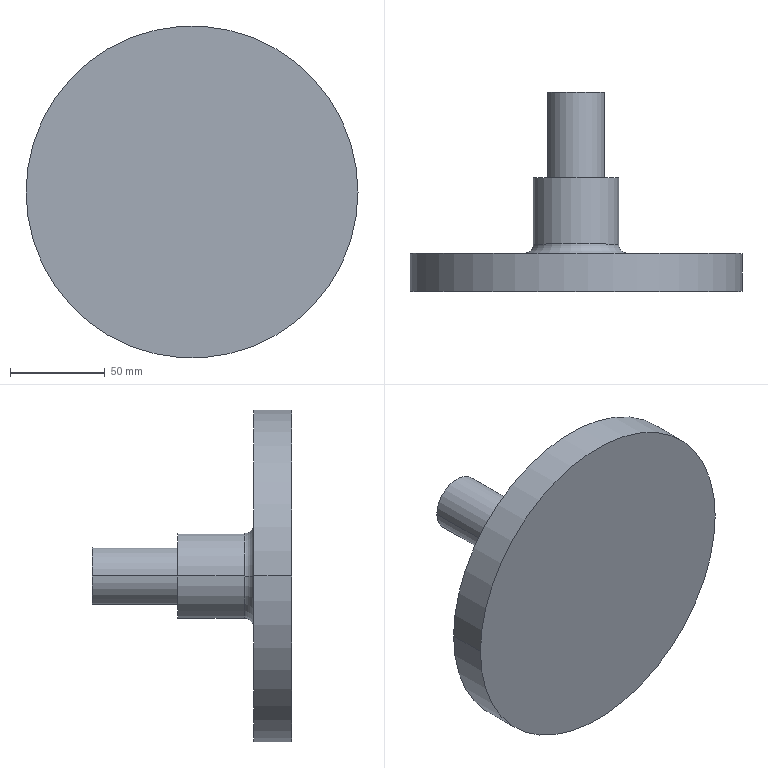Part | STEP file | Roller XG2 | 1 solid | 12 faces | box 175 x 105 x 175 mm | volume 577278 mm3 | cylinder 6 | plane 4 | torus 2 | commonest cylinder face diameters 30 x2 45 x2 175 x2
STEP:
#1=CARTESIAN_POINT('',(0.,0.,0.));
#2=DIRECTION('',(0.,0.,1.));
#3=DIRECTION('',(1.,0.,0.));
#4=AXIS2_PLACEMENT_3D('',#1,#2,#3);
#5=CARTESIAN_POINT('',(-22.5,25.,0.));
#6=VERTEX_POINT('',#5);
#7=CARTESIAN_POINT('',(-27.5,20.,0.));
#8=VERTEX_POINT('',#7);
#9=CARTESIAN_POINT('',(-27.5,25.,0.));
#10=DIRECTION('',(0.,0.,-1.));
#11=DIRECTION('',(-1.,0.,0.));
#12=AXIS2_PLACEMENT_3D('',#9,#10,#11);
#13=CIRCLE('',#12,5.);
#14=CARTESIAN_POINT('',(0.,25.,0.));
#15=DIRECTION('',(0.,1.,0.));
#16=DIRECTION('',(-1.,0.,0.));
#17=AXIS2_PLACEMENT_3D('',#14,#15,#16);
#18=TOROIDAL_SURFACE('',#17,27.5,5.);
#19=CARTESIAN_POINT('',(6.283,0.));
#20=DIRECTION('',(0.,1.));
#21=VECTOR('',#20,1.);
#22=LINE('',#19,#21);
#23=(GEOMETRIC_REPRESENTATION_CONTEXT(2)PARAMETRIC_REPRESENTATION_CONTEXT()REPRESENTATION_CONTEXT('',''));
#24=DEFINITIONAL_REPRESENTATION('',(#22),#23);
#25=PCURVE('',#18,#24);
#26=CARTESIAN_POINT('',(0.,25.,0.));
#27=DIRECTION('',(0.,1.,0.));
#28=DIRECTION('',(-1.,0.,0.));
#29=AXIS2_PLACEMENT_3D('',#26,#27,#28);
#30=TOROIDAL_SURFACE('',#29,27.5,5.);
#31=CARTESIAN_POINT('',(0.,0.));
#32=DIRECTION('',(0.,1.));
#33=VECTOR('',#32,1.);
#34=LINE('',#31,#33);
#35=(GEOMETRIC_REPRESENTATION_CONTEXT(2)PARAMETRIC_REPRESENTATION_CONTEXT()REPRESENTATION_CONTEXT('',''));
#36=DEFINITIONAL_REPRESENTATION('',(#34),#35);
#37=PCURVE('',#30,#36);
#38=SURFACE_CURVE('',#13,(#25,#37),.PCURVE_S1.);
#39=EDGE_CURVE('',#6,#8,#38,.T.);
#40=ORIENTED_EDGE('',*,*,#39,.T.);
#41=CARTESIAN_POINT('',(27.5,20.,0.));
#42=VERTEX_POINT('',#41);
#43=CARTESIAN_POINT('',(0.,20.,0.));
#44=DIRECTION('',(0.,-1.,0.));
#45=DIRECTION('',(-1.,0.,0.));
#46=AXIS2_PLACEMENT_3D('',#43,#44,#45);
#47=CIRCLE('',#46,27.5);
#48=CARTESIAN_POINT('',(6.283,4.712));
#49=DIRECTION('',(-1.,0.));
#50=VECTOR('',#49,1.);
#51=LINE('',#48,#50);
#52=(GEOMETRIC_REPRESENTATION_CONTEXT(2)PARAMETRIC_REPRESENTATION_CONTEXT()REPRESENTATION_CONTEXT('',''));
#53=DEFINITIONAL_REPRESENTATION('',(#51),#52);
#54=PCURVE('',#18,#53);
#55=CARTESIAN_POINT('',(87.5,20.,0.));
#56=DIRECTION('',(0.,1.,0.));
#57=DIRECTION('',(-1.,0.,0.));
#58=AXIS2_PLACEMENT_3D('',#55,#56,#57);
#59=PLANE('',#58);
#60=CARTESIAN_POINT('',(115.,0.));
#61=CARTESIAN_POINT('',(115.,-47.631));
#62=CARTESIAN_POINT('',(73.75,-23.816));
#63=CARTESIAN_POINT('',(32.5,0.));
#64=CARTESIAN_POINT('',(73.75,23.816));
#65=CARTESIAN_POINT('',(115.,47.631));
#66=CARTESIAN_POINT('',(115.,0.));
#67=(BOUNDED_CURVE()B_SPLINE_CURVE(2,(#60,#61,#62,#63,#64,#65,#66),.UNSPECIFIED.,.T.,.F.)B_SPLINE_CURVE_WITH_KNOTS((1,2,2,2,2,1),(-2.094,0.,2.094,4.189,6.283,8.378),.UNSPECIFIED.)CURVE()GEOMETRIC_REPRESENTATION_ITEM()RATIONAL_B_SPLINE_CURVE((1.,0.5,1.,0.5,1.,0.5,1.))REPRESENTATION_ITEM(''));
#68=(GEOMETRIC_REPRESENTATION_CONTEXT(2)PARAMETRIC_REPRESENTATION_CONTEXT()REPRESENTATION_CONTEXT('',''));
#69=DEFINITIONAL_REPRESENTATION('',(#67),#68);
#70=PCURVE('',#59,#69);
#71=SURFACE_CURVE('',#47,(#54,#70),.PCURVE_S1.);
#72=EDGE_CURVE('',#8,#42,#71,.T.);
#73=ORIENTED_EDGE('',*,*,#72,.T.);
#74=CARTESIAN_POINT('',(22.5,25.,0.));
#75=VERTEX_POINT('',#74);
#76=CARTESIAN_POINT('',(27.5,25.,0.));
#77=DIRECTION('',(0.,0.,1.));
#78=DIRECTION('',(1.,0.,0.));
#79=AXIS2_PLACEMENT_3D('',#76,#77,#78);
#80=CIRCLE('',#79,5.);
#81=CARTESIAN_POINT('',(3.142,0.));
#82=DIRECTION('',(0.,1.));
#83=VECTOR('',#82,1.);
#84=LINE('',#81,#83);
#85=(GEOMETRIC_REPRESENTATION_CONTEXT(2)PARAMETRIC_REPRESENTATION_CONTEXT()REPRESENTATION_CONTEXT('',''));
#86=DEFINITIONAL_REPRESENTATION('',(#84),#85);
#87=PCURVE('',#18,#86);
#88=CARTESIAN_POINT('',(3.142,0.));
#89=DIRECTION('',(0.,1.));
#90=VECTOR('',#89,1.);
#91=LINE('',#88,#90);
#92=(GEOMETRIC_REPRESENTATION_CONTEXT(2)PARAMETRIC_REPRESENTATION_CONTEXT()REPRESENTATION_CONTEXT('',''));
#93=DEFINITIONAL_REPRESENTATION('',(#91),#92);
#94=PCURVE('',#30,#93);
#95=SURFACE_CURVE('',#80,(#87,#94),.PCURVE_S1.);
#96=EDGE_CURVE('',#75,#42,#95,.T.);
#97=ORIENTED_EDGE('',*,*,#96,.F.);
#98=CARTESIAN_POINT('',(0.,25.,0.));
#99=DIRECTION('',(0.,1.,0.));
#100=DIRECTION('',(-1.,0.,0.));
#101=AXIS2_PLACEMENT_3D('',#98,#99,#100);
#102=CIRCLE('',#101,22.5);
#103=CARTESIAN_POINT('',(0.,3.142));
#104=DIRECTION('',(1.,0.));
#105=VECTOR('',#104,1.);
#106=LINE('',#103,#105);
#107=(GEOMETRIC_REPRESENTATION_CONTEXT(2)PARAMETRIC_REPRESENTATION_CONTEXT()REPRESENTATION_CONTEXT('',''));
#108=DEFINITIONAL_REPRESENTATION('',(#106),#107);
#109=PCURVE('',#18,#108);
#110=CARTESIAN_POINT('',(0.,-777.265,0.));
#111=DIRECTION('',(0.,-1.,0.));
#112=DIRECTION('',(1.,0.,0.));
#113=AXIS2_PLACEMENT_3D('',#110,#111,#112);
#114=CYLINDRICAL_SURFACE('',#113,22.5);
#115=CARTESIAN_POINT('',(9.425,-802.265));
#116=DIRECTION('',(-1.,0.));
#117=VECTOR('',#116,1.);
#118=LINE('',#115,#117);
#119=(GEOMETRIC_REPRESENTATION_CONTEXT(2)PARAMETRIC_REPRESENTATION_CONTEXT()REPRESENTATION_CONTEXT('',''));
#120=DEFINITIONAL_REPRESENTATION('',(#118),#119);
#121=PCURVE('',#114,#120);
#122=SURFACE_CURVE('',#102,(#109,#121),.PCURVE_S1.);
#123=EDGE_CURVE('',#75,#6,#122,.T.);
#124=ORIENTED_EDGE('',*,*,#123,.T.);
#125=EDGE_LOOP('',(#40,#73,#97,#124));
#126=FACE_BOUND('',#125,.F.);
#127=ADVANCED_FACE('',(#126),#18,.F.);
#128=CARTESIAN_POINT('',(15.,105.,0.));
#129=VERTEX_POINT('',#128);
#130=CARTESIAN_POINT('',(-15.,105.,0.));
#131=VERTEX_POINT('',#130);
#132=CARTESIAN_POINT('',(0.,105.,0.));
#133=DIRECTION('',(0.,-1.,0.));
#134=DIRECTION('',(1.,0.,0.));
#135=AXIS2_PLACEMENT_3D('',#132,#133,#134);
#136=CIRCLE('',#135,15.);
#137=CARTESIAN_POINT('',(0.,-777.265,0.));
#138=DIRECTION('',(0.,-1.,0.));
#139=DIRECTION('',(1.,0.,0.));
#140=AXIS2_PLACEMENT_3D('',#137,#138,#139);
#141=CYLINDRICAL_SURFACE('',#140,15.);
#142=CARTESIAN_POINT('',(0.,-882.265));
#143=DIRECTION('',(1.,0.));
#144=VECTOR('',#143,1.);
#145=LINE('',#142,#144);
#146=(GEOMETRIC_REPRESENTATION_CONTEXT(2)PARAMETRIC_REPRESENTATION_CONTEXT()REPRESENTATION_CONTEXT('',''));
#147=DEFINITIONAL_REPRESENTATION('',(#145),#146);
#148=PCURVE('',#141,#147);
#149=CARTESIAN_POINT('',(15.,105.,0.));
#150=DIRECTION('',(0.,1.,0.));
#151=DIRECTION('',(-1.,0.,0.));
#152=AXIS2_PLACEMENT_3D('',#149,#150,#151);
#153=PLANE('',#152);
#154=CARTESIAN_POINT('',(0.,0.));
#155=CARTESIAN_POINT('',(0.,25.981));
#156=CARTESIAN_POINT('',(22.5,12.99));
#157=CARTESIAN_POINT('',(45.,0.));
#158=CARTESIAN_POINT('',(22.5,-12.99));
#159=CARTESIAN_POINT('',(0.,-25.981));
#160=CARTESIAN_POINT('',(0.,0.));
#161=(BOUNDED_CURVE()B_SPLINE_CURVE(2,(#154,#155,#156,#157,#158,#159,#160),.UNSPECIFIED.,.T.,.F.)B_SPLINE_CURVE_WITH_KNOTS((1,2,2,2,2,1),(-2.094,0.,2.094,4.189,6.283,8.378),.UNSPECIFIED.)CURVE()GEOMETRIC_REPRESENTATION_ITEM()RATIONAL_B_SPLINE_CURVE((1.,0.5,1.,0.5,1.,0.5,1.))REPRESENTATION_ITEM(''));
#162=(GEOMETRIC_REPRESENTATION_CONTEXT(2)PARAMETRIC_REPRESENTATION_CONTEXT()REPRESENTATION_CONTEXT('',''));
#163=DEFINITIONAL_REPRESENTATION('',(#161),#162);
#164=PCURVE('',#153,#163);
#165=SURFACE_CURVE('',#136,(#148,#164),.PCURVE_S1.);
#166=EDGE_CURVE('',#129,#131,#165,.T.);
#167=ORIENTED_EDGE('',*,*,#166,.T.);
#168=CARTESIAN_POINT('',(-15.,60.,0.));
#169=VERTEX_POINT('',#168);
#170=CARTESIAN_POINT('',(-15.,-777.265,0.));
#171=DIRECTION('',(0.,-1.,0.));
#172=VECTOR('',#171,1.);
#173=LINE('',#170,#172);
#174=CARTESIAN_POINT('',(3.142,0.));
#175=DIRECTION('',(0.,1.));
#176=VECTOR('',#175,1.);
#177=LINE('',#174,#176);
#178=(GEOMETRIC_REPRESENTATION_CONTEXT(2)PARAMETRIC_REPRESENTATION_CONTEXT()REPRESENTATION_CONTEXT('',''));
#179=DEFINITIONAL_REPRESENTATION('',(#177),#178);
#180=PCURVE('',#141,#179);
#181=CARTESIAN_POINT('',(0.,-777.265,0.));
#182=DIRECTION('',(0.,-1.,0.));
#183=DIRECTION('',(1.,0.,0.));
#184=AXIS2_PLACEMENT_3D('',#181,#182,#183);
#185=CYLINDRICAL_SURFACE('',#184,15.);
#186=CARTESIAN_POINT('',(3.142,0.));
#187=DIRECTION('',(0.,1.));
#188=VECTOR('',#187,1.);
#189=LINE('',#186,#188);
#190=(GEOMETRIC_REPRESENTATION_CONTEXT(2)PARAMETRIC_REPRESENTATION_CONTEXT()REPRESENTATION_CONTEXT('',''));
#191=DEFINITIONAL_REPRESENTATION('',(#189),#190);
#192=PCURVE('',#185,#191);
#193=SURFACE_CURVE('',#173,(#180,#192),.PCURVE_S1.);
#194=EDGE_CURVE('',#131,#169,#193,.T.);
#195=ORIENTED_EDGE('',*,*,#194,.T.);
#196=CARTESIAN_POINT('',(15.,60.,0.));
#197=VERTEX_POINT('',#196);
#198=CARTESIAN_POINT('',(0.,60.,0.));
#199=DIRECTION('',(0.,-1.,0.));
#200=DIRECTION('',(1.,0.,0.));
#201=AXIS2_PLACEMENT_3D('',#198,#199,#200);
#202=CIRCLE('',#201,15.);
#203=CARTESIAN_POINT('',(0.,-837.265));
#204=DIRECTION('',(1.,0.));
#205=VECTOR('',#204,1.);
#206=LINE('',#203,#205);
#207=(GEOMETRIC_REPRESENTATION_CONTEXT(2)PARAMETRIC_REPRESENTATION_CONTEXT()REPRESENTATION_CONTEXT('',''));
#208=DEFINITIONAL_REPRESENTATION('',(#206),#207);
#209=PCURVE('',#141,#208);
#210=CARTESIAN_POINT('',(22.5,60.,0.));
#211=DIRECTION('',(0.,1.,0.));
#212=DIRECTION('',(-1.,0.,0.));
#213=AXIS2_PLACEMENT_3D('',#210,#211,#212);
#214=PLANE('',#213);
#215=CARTESIAN_POINT('',(7.5,0.));
#216=CARTESIAN_POINT('',(7.5,25.981));
#217=CARTESIAN_POINT('',(30.,12.99));
#218=CARTESIAN_POINT('',(52.5,0.));
#219=CARTESIAN_POINT('',(30.,-12.99));
#220=CARTESIAN_POINT('',(7.5,-25.981));
#221=CARTESIAN_POINT('',(7.5,0.));
#222=(BOUNDED_CURVE()B_SPLINE_CURVE(2,(#215,#216,#217,#218,#219,#220,#221),.UNSPECIFIED.,.T.,.F.)B_SPLINE_CURVE_WITH_KNOTS((1,2,2,2,2,1),(-2.094,0.,2.094,4.189,6.283,8.378),.UNSPECIFIED.)CURVE()GEOMETRIC_REPRESENTATION_ITEM()RATIONAL_B_SPLINE_CURVE((1.,0.5,1.,0.5,1.,0.5,1.))REPRESENTATION_ITEM(''));
#223=(GEOMETRIC_REPRESENTATION_CONTEXT(2)PARAMETRIC_REPRESENTATION_CONTEXT()REPRESENTATION_CONTEXT('',''));
#224=DEFINITIONAL_REPRESENTATION('',(#222),#223);
#225=PCURVE('',#214,#224);
#226=SURFACE_CURVE('',#202,(#209,#225),.PCURVE_S1.);
#227=EDGE_CURVE('',#197,#169,#226,.T.);
#228=ORIENTED_EDGE('',*,*,#227,.F.);
#229=CARTESIAN_POINT('',(15.,-777.265,0.));
#230=DIRECTION('',(0.,-1.,0.));
#231=VECTOR('',#230,1.);
#232=LINE('',#229,#231);
#233=CARTESIAN_POINT('',(0.,0.));
#234=DIRECTION('',(0.,1.));
#235=VECTOR('',#234,1.);
#236=LINE('',#233,#235);
#237=(GEOMETRIC_REPRESENTATION_CONTEXT(2)PARAMETRIC_REPRESENTATION_CONTEXT()REPRESENTATION_CONTEXT('',''));
#238=DEFINITIONAL_REPRESENTATION('',(#236),#237);
#239=PCURVE('',#141,#238);
#240=CARTESIAN_POINT('',(6.283,0.));
#241=DIRECTION('',(0.,1.));
#242=VECTOR('',#241,1.);
#243=LINE('',#240,#242);
#244=(GEOMETRIC_REPRESENTATION_CONTEXT(2)PARAMETRIC_REPRESENTATION_CONTEXT()REPRESENTATION_CONTEXT('',''));
#245=DEFINITIONAL_REPRESENTATION('',(#243),#244);
#246=PCURVE('',#185,#245);
#247=SURFACE_CURVE('',#232,(#239,#246),.PCURVE_S1.);
#248=EDGE_CURVE('',#129,#197,#247,.T.);
#249=ORIENTED_EDGE('',*,*,#248,.F.);
#250=EDGE_LOOP('',(#167,#195,#228,#249));
#251=FACE_BOUND('',#250,.T.);
#252=ADVANCED_FACE('',(#251),#141,.T.);
#253=CARTESIAN_POINT('',(22.5,60.,0.));
#254=VERTEX_POINT('',#253);
#255=CARTESIAN_POINT('',(-22.5,60.,0.));
#256=VERTEX_POINT('',#255);
#257=CARTESIAN_POINT('',(0.,60.,0.));
#258=DIRECTION('',(0.,-1.,0.));
#259=DIRECTION('',(1.,0.,0.));
#260=AXIS2_PLACEMENT_3D('',#257,#258,#259);
#261=CIRCLE('',#260,22.5);
#262=CARTESIAN_POINT('',(0.,-777.265,0.));
#263=DIRECTION('',(0.,-1.,0.));
#264=DIRECTION('',(1.,0.,0.));
#265=AXIS2_PLACEMENT_3D('',#262,#263,#264);
#266=CYLINDRICAL_SURFACE('',#265,22.5);
#267=CARTESIAN_POINT('',(0.,-837.265));
#268=DIRECTION('',(1.,0.));
#269=VECTOR('',#268,1.);
#270=LINE('',#267,#269);
#271=(GEOMETRIC_REPRESENTATION_CONTEXT(2)PARAMETRIC_REPRESENTATION_CONTEXT()REPRESENTATION_CONTEXT('',''));
#272=DEFINITIONAL_REPRESENTATION('',(#270),#271);
#273=PCURVE('',#266,#272);
#274=CARTESIAN_POINT('',(0.,0.));
#275=CARTESIAN_POINT('',(0.,38.971));
#276=CARTESIAN_POINT('',(33.75,19.486));
#277=CARTESIAN_POINT('',(67.5,0.));
#278=CARTESIAN_POINT('',(33.75,-19.486));
#279=CARTESIAN_POINT('',(0.,-38.971));
#280=CARTESIAN_POINT('',(0.,0.));
#281=(BOUNDED_CURVE()B_SPLINE_CURVE(2,(#274,#275,#276,#277,#278,#279,#280),.UNSPECIFIED.,.T.,.F.)B_SPLINE_CURVE_WITH_KNOTS((1,2,2,2,2,1),(-2.094,0.,2.094,4.189,6.283,8.378),.UNSPECIFIED.)CURVE()GEOMETRIC_REPRESENTATION_ITEM()RATIONAL_B_SPLINE_CURVE((1.,0.5,1.,0.5,1.,0.5,1.))REPRESENTATION_ITEM(''));
#282=(GEOMETRIC_REPRESENTATION_CONTEXT(2)PARAMETRIC_REPRESENTATION_CONTEXT()REPRESENTATION_CONTEXT('',''));
#283=DEFINITIONAL_REPRESENTATION('',(#281),#282);
#284=PCURVE('',#214,#283);
#285=SURFACE_CURVE('',#261,(#273,#284),.PCURVE_S1.);
#286=EDGE_CURVE('',#254,#256,#285,.T.);
#287=ORIENTED_EDGE('',*,*,#286,.T.);
#288=CARTESIAN_POINT('',(-22.5,-777.265,0.));
#289=DIRECTION('',(0.,-1.,0.));
#290=VECTOR('',#289,1.);
#291=LINE('',#288,#290);
#292=CARTESIAN_POINT('',(3.142,0.));
#293=DIRECTION('',(0.,1.));
#294=VECTOR('',#293,1.);
#295=LINE('',#292,#294);
#296=(GEOMETRIC_REPRESENTATION_CONTEXT(2)PARAMETRIC_REPRESENTATION_CONTEXT()REPRESENTATION_CONTEXT('',''));
#297=DEFINITIONAL_REPRESENTATION('',(#295),#296);
#298=PCURVE('',#266,#297);
#299=CARTESIAN_POINT('',(3.142,0.));
#300=DIRECTION('',(0.,1.));
#301=VECTOR('',#300,1.);
#302=LINE('',#299,#301);
#303=(GEOMETRIC_REPRESENTATION_CONTEXT(2)PARAMETRIC_REPRESENTATION_CONTEXT()REPRESENTATION_CONTEXT('',''));
#304=DEFINITIONAL_REPRESENTATION('',(#302),#303);
#305=PCURVE('',#114,#304);
#306=SURFACE_CURVE('',#291,(#298,#305),.PCURVE_S1.);
#307=EDGE_CURVE('',#256,#6,#306,.T.);
#308=ORIENTED_EDGE('',*,*,#307,.T.);
#309=CARTESIAN_POINT('',(0.,25.,0.));
#310=DIRECTION('',(0.,1.,0.));
#311=DIRECTION('',(-1.,0.,0.));
#312=AXIS2_PLACEMENT_3D('',#309,#310,#311);
#313=CIRCLE('',#312,22.5);
#314=CARTESIAN_POINT('',(3.142,-802.265));
#315=DIRECTION('',(-1.,0.));
#316=VECTOR('',#315,1.);
#317=LINE('',#314,#316);
#318=(GEOMETRIC_REPRESENTATION_CONTEXT(2)PARAMETRIC_REPRESENTATION_CONTEXT()REPRESENTATION_CONTEXT('',''));
#319=DEFINITIONAL_REPRESENTATION('',(#317),#318);
#320=PCURVE('',#266,#319);
#321=CARTESIAN_POINT('',(0.,3.142));
#322=DIRECTION('',(1.,0.));
#323=VECTOR('',#322,1.);
#324=LINE('',#321,#323);
#325=(GEOMETRIC_REPRESENTATION_CONTEXT(2)PARAMETRIC_REPRESENTATION_CONTEXT()REPRESENTATION_CONTEXT('',''));
#326=DEFINITIONAL_REPRESENTATION('',(#324),#325);
#327=PCURVE('',#30,#326);
#328=SURFACE_CURVE('',#313,(#320,#327),.PCURVE_S1.);
#329=EDGE_CURVE('',#6,#75,#328,.T.);
#330=ORIENTED_EDGE('',*,*,#329,.T.);
#331=CARTESIAN_POINT('',(22.5,-777.265,0.));
#332=DIRECTION('',(0.,-1.,0.));
#333=VECTOR('',#332,1.);
#334=LINE('',#331,#333);
#335=CARTESIAN_POINT('',(0.,0.));
#336=DIRECTION('',(0.,1.));
#337=VECTOR('',#336,1.);
#338=LINE('',#335,#337);
#339=(GEOMETRIC_REPRESENTATION_CONTEXT(2)PARAMETRIC_REPRESENTATION_CONTEXT()REPRESENTATION_CONTEXT('',''));
#340=DEFINITIONAL_REPRESENTATION('',(#338),#339);
#341=PCURVE('',#266,#340);
#342=CARTESIAN_POINT('',(6.283,0.));
#343=DIRECTION('',(0.,1.));
#344=VECTOR('',#343,1.);
#345=LINE('',#342,#344);
#346=(GEOMETRIC_REPRESENTATION_CONTEXT(2)PARAMETRIC_REPRESENTATION_CONTEXT()REPRESENTATION_CONTEXT('',''));
#347=DEFINITIONAL_REPRESENTATION('',(#345),#346);
#348=PCURVE('',#114,#347);
#349=SURFACE_CURVE('',#334,(#341,#348),.PCURVE_S1.);
#350=EDGE_CURVE('',#254,#75,#349,.T.);
#351=ORIENTED_EDGE('',*,*,#350,.F.);
#352=EDGE_LOOP('',(#287,#308,#330,#351));
#353=FACE_BOUND('',#352,.T.);
#354=ADVANCED_FACE('',(#353),#266,.T.);
#355=CARTESIAN_POINT('',(87.5,20.,0.));
#356=VERTEX_POINT('',#355);
#357=CARTESIAN_POINT('',(-87.5,20.,0.));
#358=VERTEX_POINT('',#357);
#359=CARTESIAN_POINT('',(0.,20.,0.));
#360=DIRECTION('',(0.,-1.,0.));
#361=DIRECTION('',(1.,0.,0.));
#362=AXIS2_PLACEMENT_3D('',#359,#360,#361);
#363=CIRCLE('',#362,87.5);
#364=CARTESIAN_POINT('',(0.,-777.265,0.));
#365=DIRECTION('',(0.,-1.,0.));
#366=DIRECTION('',(1.,0.,0.));
#367=AXIS2_PLACEMENT_3D('',#364,#365,#366);
#368=CYLINDRICAL_SURFACE('',#367,87.5);
#369=CARTESIAN_POINT('',(0.,-797.265));
#370=DIRECTION('',(1.,0.));
#371=VECTOR('',#370,1.);
#372=LINE('',#369,#371);
#373=(GEOMETRIC_REPRESENTATION_CONTEXT(2)PARAMETRIC_REPRESENTATION_CONTEXT()REPRESENTATION_CONTEXT('',''));
#374=DEFINITIONAL_REPRESENTATION('',(#372),#373);
#375=PCURVE('',#368,#374);
#376=CARTESIAN_POINT('',(0.,0.));
#377=CARTESIAN_POINT('',(0.,151.554));
#378=CARTESIAN_POINT('',(131.25,75.777));
#379=CARTESIAN_POINT('',(262.5,0.));
#380=CARTESIAN_POINT('',(131.25,-75.777));
#381=CARTESIAN_POINT('',(0.,-151.554));
#382=CARTESIAN_POINT('',(0.,0.));
#383=(BOUNDED_CURVE()B_SPLINE_CURVE(2,(#376,#377,#378,#379,#380,#381,#382),.UNSPECIFIED.,.T.,.F.)B_SPLINE_CURVE_WITH_KNOTS((1,2,2,2,2,1),(-2.094,0.,2.094,4.189,6.283,8.378),.UNSPECIFIED.)CURVE()GEOMETRIC_REPRESENTATION_ITEM()RATIONAL_B_SPLINE_CURVE((1.,0.5,1.,0.5,1.,0.5,1.))REPRESENTATION_ITEM(''));
#384=(GEOMETRIC_REPRESENTATION_CONTEXT(2)PARAMETRIC_REPRESENTATION_CONTEXT()REPRESENTATION_CONTEXT('',''));
#385=DEFINITIONAL_REPRESENTATION('',(#383),#384);
#386=PCURVE('',#59,#385);
#387=SURFACE_CURVE('',#363,(#375,#386),.PCURVE_S1.);
#388=EDGE_CURVE('',#356,#358,#387,.T.);
#389=ORIENTED_EDGE('',*,*,#388,.T.);
#390=CARTESIAN_POINT('',(-87.5,0.,0.));
#391=VERTEX_POINT('',#390);
#392=CARTESIAN_POINT('',(-87.5,-777.265,0.));
#393=DIRECTION('',(0.,-1.,0.));
#394=VECTOR('',#393,1.);
#395=LINE('',#392,#394);
#396=CARTESIAN_POINT('',(3.142,0.));
#397=DIRECTION('',(0.,1.));
#398=VECTOR('',#397,1.);
#399=LINE('',#396,#398);
#400=(GEOMETRIC_REPRESENTATION_CONTEXT(2)PARAMETRIC_REPRESENTATION_CONTEXT()REPRESENTATION_CONTEXT('',''));
#401=DEFINITIONAL_REPRESENTATION('',(#399),#400);
#402=PCURVE('',#368,#401);
#403=CARTESIAN_POINT('',(0.,-777.265,0.));
#404=DIRECTION('',(0.,-1.,0.));
#405=DIRECTION('',(1.,0.,0.));
#406=AXIS2_PLACEMENT_3D('',#403,#404,#405);
#407=CYLINDRICAL_SURFACE('',#406,87.5);
#408=CARTESIAN_POINT('',(3.142,0.));
#409=DIRECTION('',(0.,1.));
#410=VECTOR('',#409,1.);
#411=LINE('',#408,#410);
#412=(GEOMETRIC_REPRESENTATION_CONTEXT(2)PARAMETRIC_REPRESENTATION_CONTEXT()REPRESENTATION_CONTEXT('',''));
#413=DEFINITIONAL_REPRESENTATION('',(#411),#412);
#414=PCURVE('',#407,#413);
#415=SURFACE_CURVE('',#395,(#402,#414),.PCURVE_S1.);
#416=EDGE_CURVE('',#358,#391,#415,.T.);
#417=ORIENTED_EDGE('',*,*,#416,.T.);
#418=CARTESIAN_POINT('',(87.5,0.,0.));
#419=VERTEX_POINT('',#418);
#420=CARTESIAN_POINT('',(0.,0.,0.));
#421=DIRECTION('',(0.,-1.,0.));
#422=DIRECTION('',(1.,0.,0.));
#423=AXIS2_PLACEMENT_3D('',#420,#421,#422);
#424=CIRCLE('',#423,87.5);
#425=CARTESIAN_POINT('',(0.,-777.265));
#426=DIRECTION('',(1.,0.));
#427=VECTOR('',#426,1.);
#428=LINE('',#425,#427);
#429=(GEOMETRIC_REPRESENTATION_CONTEXT(2)PARAMETRIC_REPRESENTATION_CONTEXT()REPRESENTATION_CONTEXT('',''));
#430=DEFINITIONAL_REPRESENTATION('',(#428),#429);
#431=PCURVE('',#368,#430);
#432=CARTESIAN_POINT('',(87.5,0.,0.));
#433=DIRECTION('',(0.,-1.,0.));
#434=DIRECTION('',(1.,0.,0.));
#435=AXIS2_PLACEMENT_3D('',#432,#433,#434);
#436=PLANE('',#435);
#437=CARTESIAN_POINT('',(-87.5,0.));
#438=DIRECTION('',(1.,0.));
#439=AXIS2_PLACEMENT_2D('',#437,#438);
#440=CIRCLE('',#439,87.5);
#441=(GEOMETRIC_REPRESENTATION_CONTEXT(2)PARAMETRIC_REPRESENTATION_CONTEXT()REPRESENTATION_CONTEXT('',''));
#442=DEFINITIONAL_REPRESENTATION('',(#440),#441);
#443=PCURVE('',#436,#442);
#444=SURFACE_CURVE('',#424,(#431,#443),.PCURVE_S1.);
#445=EDGE_CURVE('',#419,#391,#444,.T.);
#446=ORIENTED_EDGE('',*,*,#445,.F.);
#447=CARTESIAN_POINT('',(87.5,-777.265,0.));
#448=DIRECTION('',(0.,-1.,0.));
#449=VECTOR('',#448,1.);
#450=LINE('',#447,#449);
#451=CARTESIAN_POINT('',(0.,0.));
#452=DIRECTION('',(0.,1.));
#453=VECTOR('',#452,1.);
#454=LINE('',#451,#453);
#455=(GEOMETRIC_REPRESENTATION_CONTEXT(2)PARAMETRIC_REPRESENTATION_CONTEXT()REPRESENTATION_CONTEXT('',''));
#456=DEFINITIONAL_REPRESENTATION('',(#454),#455);
#457=PCURVE('',#368,#456);
#458=CARTESIAN_POINT('',(6.283,0.));
#459=DIRECTION('',(0.,1.));
#460=VECTOR('',#459,1.);
#461=LINE('',#458,#460);
#462=(GEOMETRIC_REPRESENTATION_CONTEXT(2)PARAMETRIC_REPRESENTATION_CONTEXT()REPRESENTATION_CONTEXT('',''));
#463=DEFINITIONAL_REPRESENTATION('',(#461),#462);
#464=PCURVE('',#407,#463);
#465=SURFACE_CURVE('',#450,(#457,#464),.PCURVE_S1.);
#466=EDGE_CURVE('',#356,#419,#465,.T.);
#467=ORIENTED_EDGE('',*,*,#466,.F.);
#468=EDGE_LOOP('',(#389,#417,#446,#467));
#469=FACE_BOUND('',#468,.T.);
#470=ADVANCED_FACE('',(#469),#368,.T.);
#471=ORIENTED_EDGE('',*,*,#416,.F.);
#472=CARTESIAN_POINT('',(0.,20.,0.));
#473=DIRECTION('',(0.,-1.,0.));
#474=DIRECTION('',(1.,0.,0.));
#475=AXIS2_PLACEMENT_3D('',#472,#473,#474);
#476=CIRCLE('',#475,87.5);
#477=CARTESIAN_POINT('',(0.,-797.265));
#478=DIRECTION('',(1.,0.));
#479=VECTOR('',#478,1.);
#480=LINE('',#477,#479);
#481=(GEOMETRIC_REPRESENTATION_CONTEXT(2)PARAMETRIC_REPRESENTATION_CONTEXT()REPRESENTATION_CONTEXT('',''));
#482=DEFINITIONAL_REPRESENTATION('',(#480),#481);
#483=PCURVE('',#407,#482);
#484=CARTESIAN_POINT('',(0.,0.));
#485=CARTESIAN_POINT('',(0.,151.554));
#486=CARTESIAN_POINT('',(131.25,75.777));
#487=CARTESIAN_POINT('',(262.5,0.));
#488=CARTESIAN_POINT('',(131.25,-75.777));
#489=CARTESIAN_POINT('',(0.,-151.554));
#490=CARTESIAN_POINT('',(0.,0.));
#491=(BOUNDED_CURVE()B_SPLINE_CURVE(2,(#484,#485,#486,#487,#488,#489,#490),.UNSPECIFIED.,.T.,.F.)B_SPLINE_CURVE_WITH_KNOTS((1,2,2,2,2,1),(-2.094,0.,2.094,4.189,6.283,8.378),.UNSPECIFIED.)CURVE()GEOMETRIC_REPRESENTATION_ITEM()RATIONAL_B_SPLINE_CURVE((1.,0.5,1.,0.5,1.,0.5,1.))REPRESENTATION_ITEM(''));
#492=(GEOMETRIC_REPRESENTATION_CONTEXT(2)PARAMETRIC_REPRESENTATION_CONTEXT()REPRESENTATION_CONTEXT('',''));
#493=DEFINITIONAL_REPRESENTATION('',(#491),#492);
#494=PCURVE('',#59,#493);
#495=SURFACE_CURVE('',#476,(#483,#494),.PCURVE_S1.);
#496=EDGE_CURVE('',#358,#356,#495,.T.);
#497=ORIENTED_EDGE('',*,*,#496,.T.);
#498=ORIENTED_EDGE('',*,*,#466,.T.);
#499=CARTESIAN_POINT('',(0.,0.,0.));
#500=DIRECTION('',(0.,-1.,0.));
#501=DIRECTION('',(1.,0.,0.));
#502=AXIS2_PLACEMENT_3D('',#499,#500,#501);
#503=CIRCLE('',#502,87.5);
#504=CARTESIAN_POINT('',(0.,-777.265));
#505=DIRECTION('',(1.,0.));
#506=VECTOR('',#505,1.);
#507=LINE('',#504,#506);
#508=(GEOMETRIC_REPRESENTATION_CONTEXT(2)PARAMETRIC_REPRESENTATION_CONTEXT()REPRESENTATION_CONTEXT('',''));
#509=DEFINITIONAL_REPRESENTATION('',(#507),#508);
#510=PCURVE('',#407,#509);
#511=CARTESIAN_POINT('',(-87.5,0.));
#512=DIRECTION('',(1.,0.));
#513=AXIS2_PLACEMENT_2D('',#511,#512);
#514=CIRCLE('',#513,87.5);
#515=(GEOMETRIC_REPRESENTATION_CONTEXT(2)PARAMETRIC_REPRESENTATION_CONTEXT()REPRESENTATION_CONTEXT('',''));
#516=DEFINITIONAL_REPRESENTATION('',(#514),#515);
#517=PCURVE('',#436,#516);
#518=SURFACE_CURVE('',#503,(#510,#517),.PCURVE_S1.);
#519=EDGE_CURVE('',#391,#419,#518,.T.);
#520=ORIENTED_EDGE('',*,*,#519,.F.);
#521=EDGE_LOOP('',(#471,#497,#498,#520));
#522=FACE_BOUND('',#521,.T.);
#523=ADVANCED_FACE('',(#522),#407,.T.);
#524=ORIENTED_EDGE('',*,*,#72,.T.);
#525=CARTESIAN_POINT('',(0.,20.,0.));
#526=DIRECTION('',(0.,-1.,0.));
#527=DIRECTION('',(-1.,0.,0.));
#528=AXIS2_PLACEMENT_3D('',#525,#526,#527);
#529=CIRCLE('',#528,27.5);
#530=CARTESIAN_POINT('',(115.,0.));
#531=CARTESIAN_POINT('',(115.,-47.631));
#532=CARTESIAN_POINT('',(73.75,-23.816));
#533=CARTESIAN_POINT('',(32.5,0.));
#534=CARTESIAN_POINT('',(73.75,23.816));
#535=CARTESIAN_POINT('',(115.,47.631));
#536=CARTESIAN_POINT('',(115.,0.));
#537=(BOUNDED_CURVE()B_SPLINE_CURVE(2,(#530,#531,#532,#533,#534,#535,#536),.UNSPECIFIED.,.T.,.F.)B_SPLINE_CURVE_WITH_KNOTS((1,2,2,2,2,1),(-2.094,0.,2.094,4.189,6.283,8.378),.UNSPECIFIED.)CURVE()GEOMETRIC_REPRESENTATION_ITEM()RATIONAL_B_SPLINE_CURVE((1.,0.5,1.,0.5,1.,0.5,1.))REPRESENTATION_ITEM(''));
#538=(GEOMETRIC_REPRESENTATION_CONTEXT(2)PARAMETRIC_REPRESENTATION_CONTEXT()REPRESENTATION_CONTEXT('',''));
#539=DEFINITIONAL_REPRESENTATION('',(#537),#538);
#540=PCURVE('',#59,#539);
#541=CARTESIAN_POINT('',(6.283,4.712));
#542=DIRECTION('',(-1.,0.));
#543=VECTOR('',#542,1.);
#544=LINE('',#541,#543);
#545=(GEOMETRIC_REPRESENTATION_CONTEXT(2)PARAMETRIC_REPRESENTATION_CONTEXT()REPRESENTATION_CONTEXT('',''));
#546=DEFINITIONAL_REPRESENTATION('',(#544),#545);
#547=PCURVE('',#30,#546);
#548=SURFACE_CURVE('',#529,(#540,#547),.PCURVE_S1.);
#549=EDGE_CURVE('',#42,#8,#548,.T.);
#550=ORIENTED_EDGE('',*,*,#549,.T.);
#551=EDGE_LOOP('',(#524,#550));
#552=FACE_BOUND('',#551,.T.);
#553=ORIENTED_EDGE('',*,*,#388,.F.);
#554=ORIENTED_EDGE('',*,*,#496,.F.);
#555=EDGE_LOOP('',(#553,#554));
#556=FACE_BOUND('',#555,.T.);
#557=ADVANCED_FACE('',(#552,#556),#59,.T.);
#558=ORIENTED_EDGE('',*,*,#307,.F.);
#559=CARTESIAN_POINT('',(0.,60.,0.));
#560=DIRECTION('',(0.,-1.,0.));
#561=DIRECTION('',(1.,0.,0.));
#562=AXIS2_PLACEMENT_3D('',#559,#560,#561);
#563=CIRCLE('',#562,22.5);
#564=CARTESIAN_POINT('',(0.,-837.265));
#565=DIRECTION('',(1.,0.));
#566=VECTOR('',#565,1.);
#567=LINE('',#564,#566);
#568=(GEOMETRIC_REPRESENTATION_CONTEXT(2)PARAMETRIC_REPRESENTATION_CONTEXT()REPRESENTATION_CONTEXT('',''));
#569=DEFINITIONAL_REPRESENTATION('',(#567),#568);
#570=PCURVE('',#114,#569);
#571=CARTESIAN_POINT('',(0.,0.));
#572=CARTESIAN_POINT('',(0.,38.971));
#573=CARTESIAN_POINT('',(33.75,19.486));
#574=CARTESIAN_POINT('',(67.5,0.));
#575=CARTESIAN_POINT('',(33.75,-19.486));
#576=CARTESIAN_POINT('',(0.,-38.971));
#577=CARTESIAN_POINT('',(0.,0.));
#578=(BOUNDED_CURVE()B_SPLINE_CURVE(2,(#571,#572,#573,#574,#575,#576,#577),.UNSPECIFIED.,.T.,.F.)B_SPLINE_CURVE_WITH_KNOTS((1,2,2,2,2,1),(-2.094,0.,2.094,4.189,6.283,8.378),.UNSPECIFIED.)CURVE()GEOMETRIC_REPRESENTATION_ITEM()RATIONAL_B_SPLINE_CURVE((1.,0.5,1.,0.5,1.,0.5,1.))REPRESENTATION_ITEM(''));
#579=(GEOMETRIC_REPRESENTATION_CONTEXT(2)PARAMETRIC_REPRESENTATION_CONTEXT()REPRESENTATION_CONTEXT('',''));
#580=DEFINITIONAL_REPRESENTATION('',(#578),#579);
#581=PCURVE('',#214,#580);
#582=SURFACE_CURVE('',#563,(#570,#581),.PCURVE_S1.);
#583=EDGE_CURVE('',#256,#254,#582,.T.);
#584=ORIENTED_EDGE('',*,*,#583,.T.);
#585=ORIENTED_EDGE('',*,*,#350,.T.);
#586=ORIENTED_EDGE('',*,*,#123,.T.);
#587=EDGE_LOOP('',(#558,#584,#585,#586));
#588=FACE_BOUND('',#587,.T.);
#589=ADVANCED_FACE('',(#588),#114,.T.);
#590=ORIENTED_EDGE('',*,*,#227,.T.);
#591=CARTESIAN_POINT('',(0.,60.,0.));
#592=DIRECTION('',(0.,-1.,0.));
#593=DIRECTION('',(1.,0.,0.));
#594=AXIS2_PLACEMENT_3D('',#591,#592,#593);
#595=CIRCLE('',#594,15.);
#596=CARTESIAN_POINT('',(7.5,0.));
#597=CARTESIAN_POINT('',(7.5,25.981));
#598=CARTESIAN_POINT('',(30.,12.99));
#599=CARTESIAN_POINT('',(52.5,0.));
#600=CARTESIAN_POINT('',(30.,-12.99));
#601=CARTESIAN_POINT('',(7.5,-25.981));
#602=CARTESIAN_POINT('',(7.5,0.));
#603=(BOUNDED_CURVE()B_SPLINE_CURVE(2,(#596,#597,#598,#599,#600,#601,#602),.UNSPECIFIED.,.T.,.F.)B_SPLINE_CURVE_WITH_KNOTS((1,2,2,2,2,1),(-2.094,0.,2.094,4.189,6.283,8.378),.UNSPECIFIED.)CURVE()GEOMETRIC_REPRESENTATION_ITEM()RATIONAL_B_SPLINE_CURVE((1.,0.5,1.,0.5,1.,0.5,1.))REPRESENTATION_ITEM(''));
#604=(GEOMETRIC_REPRESENTATION_CONTEXT(2)PARAMETRIC_REPRESENTATION_CONTEXT()REPRESENTATION_CONTEXT('',''));
#605=DEFINITIONAL_REPRESENTATION('',(#603),#604);
#606=PCURVE('',#214,#605);
#607=CARTESIAN_POINT('',(0.,-837.265));
#608=DIRECTION('',(1.,0.));
#609=VECTOR('',#608,1.);
#610=LINE('',#607,#609);
#611=(GEOMETRIC_REPRESENTATION_CONTEXT(2)PARAMETRIC_REPRESENTATION_CONTEXT()REPRESENTATION_CONTEXT('',''));
#612=DEFINITIONAL_REPRESENTATION('',(#610),#611);
#613=PCURVE('',#185,#612);
#614=SURFACE_CURVE('',#595,(#606,#613),.PCURVE_S1.);
#615=EDGE_CURVE('',#169,#197,#614,.T.);
#616=ORIENTED_EDGE('',*,*,#615,.T.);
#617=EDGE_LOOP('',(#590,#616));
#618=FACE_BOUND('',#617,.T.);
#619=ORIENTED_EDGE('',*,*,#286,.F.);
#620=ORIENTED_EDGE('',*,*,#583,.F.);
#621=EDGE_LOOP('',(#619,#620));
#622=FACE_BOUND('',#621,.T.);
#623=ADVANCED_FACE('',(#618,#622),#214,.T.);
#624=ORIENTED_EDGE('',*,*,#194,.F.);
#625=CARTESIAN_POINT('',(0.,105.,0.));
#626=DIRECTION('',(0.,-1.,0.));
#627=DIRECTION('',(1.,0.,0.));
#628=AXIS2_PLACEMENT_3D('',#625,#626,#627);
#629=CIRCLE('',#628,15.);
#630=CARTESIAN_POINT('',(0.,-882.265));
#631=DIRECTION('',(1.,0.));
#632=VECTOR('',#631,1.);
#633=LINE('',#630,#632);
#634=(GEOMETRIC_REPRESENTATION_CONTEXT(2)PARAMETRIC_REPRESENTATION_CONTEXT()REPRESENTATION_CONTEXT('',''));
#635=DEFINITIONAL_REPRESENTATION('',(#633),#634);
#636=PCURVE('',#185,#635);
#637=CARTESIAN_POINT('',(0.,0.));
#638=CARTESIAN_POINT('',(0.,25.981));
#639=CARTESIAN_POINT('',(22.5,12.99));
#640=CARTESIAN_POINT('',(45.,0.));
#641=CARTESIAN_POINT('',(22.5,-12.99));
#642=CARTESIAN_POINT('',(0.,-25.981));
#643=CARTESIAN_POINT('',(0.,0.));
#644=(BOUNDED_CURVE()B_SPLINE_CURVE(2,(#637,#638,#639,#640,#641,#642,#643),.UNSPECIFIED.,.T.,.F.)B_SPLINE_CURVE_WITH_KNOTS((1,2,2,2,2,1),(-2.094,0.,2.094,4.189,6.283,8.378),.UNSPECIFIED.)CURVE()GEOMETRIC_REPRESENTATION_ITEM()RATIONAL_B_SPLINE_CURVE((1.,0.5,1.,0.5,1.,0.5,1.))REPRESENTATION_ITEM(''));
#645=(GEOMETRIC_REPRESENTATION_CONTEXT(2)PARAMETRIC_REPRESENTATION_CONTEXT()REPRESENTATION_CONTEXT('',''));
#646=DEFINITIONAL_REPRESENTATION('',(#644),#645);
#647=PCURVE('',#153,#646);
#648=SURFACE_CURVE('',#629,(#636,#647),.PCURVE_S1.);
#649=EDGE_CURVE('',#131,#129,#648,.T.);
#650=ORIENTED_EDGE('',*,*,#649,.T.);
#651=ORIENTED_EDGE('',*,*,#248,.T.);
#652=ORIENTED_EDGE('',*,*,#615,.F.);
#653=EDGE_LOOP('',(#624,#650,#651,#652));
#654=FACE_BOUND('',#653,.T.);
#655=ADVANCED_FACE('',(#654),#185,.T.);
#656=ORIENTED_EDGE('',*,*,#166,.F.);
#657=ORIENTED_EDGE('',*,*,#649,.F.);
#658=EDGE_LOOP('',(#656,#657));
#659=FACE_BOUND('',#658,.T.);
#660=ADVANCED_FACE('',(#659),#153,.T.);
#661=ORIENTED_EDGE('',*,*,#445,.T.);
#662=ORIENTED_EDGE('',*,*,#519,.T.);
#663=EDGE_LOOP('',(#661,#662));
#664=FACE_BOUND('',#663,.T.);
#665=ADVANCED_FACE('',(#664),#436,.T.);
#666=ORIENTED_EDGE('',*,*,#549,.T.);
#667=ORIENTED_EDGE('',*,*,#39,.F.);
#668=ORIENTED_EDGE('',*,*,#329,.T.);
#669=ORIENTED_EDGE('',*,*,#96,.T.);
#670=EDGE_LOOP('',(#666,#667,#668,#669));
#671=FACE_BOUND('',#670,.F.);
#672=ADVANCED_FACE('',(#671),#30,.F.);
#673=CLOSED_SHELL('',(#127,#252,#354,#470,#523,#557,#589,#623,#655,#660,#665,#672));
#674=MANIFOLD_SOLID_BREP('',#673);
#675=(LENGTH_UNIT()NAMED_UNIT(*)SI_UNIT(.MILLI.,.METRE.));
#676=UNCERTAINTY_MEASURE_WITH_UNIT(LENGTH_MEASURE(0.0000001),#675,'','');
#677=(NAMED_UNIT(*)PLANE_ANGLE_UNIT()SI_UNIT($,.RADIAN.));
#678=(NAMED_UNIT(*)SI_UNIT($,.STERADIAN.)SOLID_ANGLE_UNIT());
#679=(GEOMETRIC_REPRESENTATION_CONTEXT(3)GLOBAL_UNCERTAINTY_ASSIGNED_CONTEXT((#676))GLOBAL_UNIT_ASSIGNED_CONTEXT((#675,#677,#678))REPRESENTATION_CONTEXT('',''));
#680=ADVANCED_BREP_SHAPE_REPRESENTATION('',(#4,#674),#679);